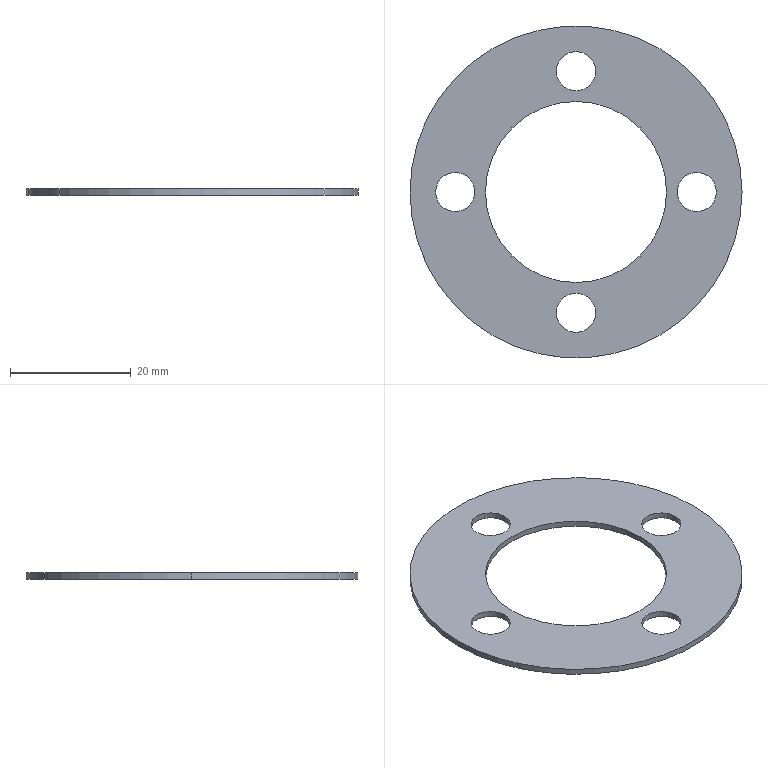Part | SolidWorks | features Extrusion 1 | 1 solid | 14 faces | box 55 x 55 x 1 mm | volume 1536 mm3 | cylinder 12 | plane 2 | commonest cylinder face diameters 6.5 x8 30 x2 55 x2
STEP:
#1=CARTESIAN_POINT('',(-23.25,0.,1.));
#2=VERTEX_POINT('',#1);
#3=CARTESIAN_POINT('',(-16.75,0.,1.));
#4=VERTEX_POINT('',#3);
#5=CARTESIAN_POINT('',(-20.,0.,1.));
#6=DIRECTION('',(0.,0.,1.));
#7=DIRECTION('',(1.,0.,0.));
#8=AXIS2_PLACEMENT_3D('',#5,#6,#7);
#9=CIRCLE('',#8,3.25);
#10=EDGE_CURVE('',#2,#4,#9,.T.);
#11=ORIENTED_EDGE('',*,*,#10,.T.);
#12=CARTESIAN_POINT('',(-16.75,0.,0.));
#13=VERTEX_POINT('',#12);
#14=CARTESIAN_POINT('',(-16.75,0.,1.));
#15=DIRECTION('',(0.,0.,-1.));
#16=VECTOR('',#15,1000.);
#17=LINE('',#14,#16);
#18=EDGE_CURVE('',#4,#13,#17,.T.);
#19=ORIENTED_EDGE('',*,*,#18,.T.);
#20=CARTESIAN_POINT('',(-23.25,0.,0.));
#21=VERTEX_POINT('',#20);
#22=CARTESIAN_POINT('',(-20.,0.,0.));
#23=DIRECTION('',(0.,0.,1.));
#24=DIRECTION('',(1.,0.,0.));
#25=AXIS2_PLACEMENT_3D('',#22,#23,#24);
#26=CIRCLE('',#25,3.25);
#27=EDGE_CURVE('',#21,#13,#26,.T.);
#28=ORIENTED_EDGE('',*,*,#27,.F.);
#29=CARTESIAN_POINT('',(-23.25,0.,1.));
#30=DIRECTION('',(0.,0.,-1.));
#31=VECTOR('',#30,1000.);
#32=LINE('',#29,#31);
#33=EDGE_CURVE('',#2,#21,#32,.T.);
#34=ORIENTED_EDGE('',*,*,#33,.F.);
#35=EDGE_LOOP('',(#11,#19,#28,#34));
#36=FACE_OUTER_BOUND('',#35,.T.);
#37=CARTESIAN_POINT('',(-20.,0.,1.));
#38=DIRECTION('',(0.,0.,-1.));
#39=DIRECTION('',(-1.,0.,0.));
#40=AXIS2_PLACEMENT_3D('',#37,#38,#39);
#41=CYLINDRICAL_SURFACE('',#40,3.25);
#42=ADVANCED_FACE('',(#36),#41,.F.);
#43=CARTESIAN_POINT('',(-3.25,-20.,1.));
#44=VERTEX_POINT('',#43);
#45=CARTESIAN_POINT('',(3.25,-20.,1.));
#46=VERTEX_POINT('',#45);
#47=CARTESIAN_POINT('',(0.,-20.,1.));
#48=DIRECTION('',(0.,0.,1.));
#49=DIRECTION('',(1.,0.,0.));
#50=AXIS2_PLACEMENT_3D('',#47,#48,#49);
#51=CIRCLE('',#50,3.25);
#52=EDGE_CURVE('',#44,#46,#51,.T.);
#53=ORIENTED_EDGE('',*,*,#52,.T.);
#54=CARTESIAN_POINT('',(3.25,-20.,0.));
#55=VERTEX_POINT('',#54);
#56=CARTESIAN_POINT('',(3.25,-20.,1.));
#57=DIRECTION('',(0.,0.,-1.));
#58=VECTOR('',#57,1000.);
#59=LINE('',#56,#58);
#60=EDGE_CURVE('',#46,#55,#59,.T.);
#61=ORIENTED_EDGE('',*,*,#60,.T.);
#62=CARTESIAN_POINT('',(-3.25,-20.,0.));
#63=VERTEX_POINT('',#62);
#64=CARTESIAN_POINT('',(0.,-20.,0.));
#65=DIRECTION('',(0.,0.,1.));
#66=DIRECTION('',(1.,0.,0.));
#67=AXIS2_PLACEMENT_3D('',#64,#65,#66);
#68=CIRCLE('',#67,3.25);
#69=EDGE_CURVE('',#63,#55,#68,.T.);
#70=ORIENTED_EDGE('',*,*,#69,.F.);
#71=CARTESIAN_POINT('',(-3.25,-20.,1.));
#72=DIRECTION('',(0.,0.,-1.));
#73=VECTOR('',#72,1000.);
#74=LINE('',#71,#73);
#75=EDGE_CURVE('',#44,#63,#74,.T.);
#76=ORIENTED_EDGE('',*,*,#75,.F.);
#77=EDGE_LOOP('',(#53,#61,#70,#76));
#78=FACE_OUTER_BOUND('',#77,.T.);
#79=CARTESIAN_POINT('',(0.,-20.,1.));
#80=DIRECTION('',(0.,0.,-1.));
#81=DIRECTION('',(-1.,0.,0.));
#82=AXIS2_PLACEMENT_3D('',#79,#80,#81);
#83=CYLINDRICAL_SURFACE('',#82,3.25);
#84=ADVANCED_FACE('',(#78),#83,.F.);
#85=CARTESIAN_POINT('',(16.75,0.,1.));
#86=VERTEX_POINT('',#85);
#87=CARTESIAN_POINT('',(23.25,0.,1.));
#88=VERTEX_POINT('',#87);
#89=CARTESIAN_POINT('',(20.,0.,1.));
#90=DIRECTION('',(0.,0.,1.));
#91=DIRECTION('',(1.,0.,0.));
#92=AXIS2_PLACEMENT_3D('',#89,#90,#91);
#93=CIRCLE('',#92,3.25);
#94=EDGE_CURVE('',#86,#88,#93,.T.);
#95=ORIENTED_EDGE('',*,*,#94,.T.);
#96=CARTESIAN_POINT('',(23.25,0.,0.));
#97=VERTEX_POINT('',#96);
#98=CARTESIAN_POINT('',(23.25,0.,1.));
#99=DIRECTION('',(0.,0.,-1.));
#100=VECTOR('',#99,1000.);
#101=LINE('',#98,#100);
#102=EDGE_CURVE('',#88,#97,#101,.T.);
#103=ORIENTED_EDGE('',*,*,#102,.T.);
#104=CARTESIAN_POINT('',(16.75,0.,0.));
#105=VERTEX_POINT('',#104);
#106=CARTESIAN_POINT('',(20.,0.,0.));
#107=DIRECTION('',(0.,0.,1.));
#108=DIRECTION('',(1.,0.,0.));
#109=AXIS2_PLACEMENT_3D('',#106,#107,#108);
#110=CIRCLE('',#109,3.25);
#111=EDGE_CURVE('',#105,#97,#110,.T.);
#112=ORIENTED_EDGE('',*,*,#111,.F.);
#113=CARTESIAN_POINT('',(16.75,0.,1.));
#114=DIRECTION('',(0.,0.,-1.));
#115=VECTOR('',#114,1000.);
#116=LINE('',#113,#115);
#117=EDGE_CURVE('',#86,#105,#116,.T.);
#118=ORIENTED_EDGE('',*,*,#117,.F.);
#119=EDGE_LOOP('',(#95,#103,#112,#118));
#120=FACE_OUTER_BOUND('',#119,.T.);
#121=CARTESIAN_POINT('',(20.,0.,1.));
#122=DIRECTION('',(0.,0.,-1.));
#123=DIRECTION('',(-1.,0.,0.));
#124=AXIS2_PLACEMENT_3D('',#121,#122,#123);
#125=CYLINDRICAL_SURFACE('',#124,3.25);
#126=ADVANCED_FACE('',(#120),#125,.F.);
#127=CARTESIAN_POINT('',(-3.25,20.,1.));
#128=VERTEX_POINT('',#127);
#129=CARTESIAN_POINT('',(3.25,20.,1.));
#130=VERTEX_POINT('',#129);
#131=CARTESIAN_POINT('',(0.,20.,1.));
#132=DIRECTION('',(0.,0.,1.));
#133=DIRECTION('',(1.,0.,0.));
#134=AXIS2_PLACEMENT_3D('',#131,#132,#133);
#135=CIRCLE('',#134,3.25);
#136=EDGE_CURVE('',#128,#130,#135,.T.);
#137=ORIENTED_EDGE('',*,*,#136,.T.);
#138=CARTESIAN_POINT('',(3.25,20.,0.));
#139=VERTEX_POINT('',#138);
#140=CARTESIAN_POINT('',(3.25,20.,1.));
#141=DIRECTION('',(0.,0.,-1.));
#142=VECTOR('',#141,1000.);
#143=LINE('',#140,#142);
#144=EDGE_CURVE('',#130,#139,#143,.T.);
#145=ORIENTED_EDGE('',*,*,#144,.T.);
#146=CARTESIAN_POINT('',(-3.25,20.,0.));
#147=VERTEX_POINT('',#146);
#148=CARTESIAN_POINT('',(0.,20.,0.));
#149=DIRECTION('',(0.,0.,1.));
#150=DIRECTION('',(1.,0.,0.));
#151=AXIS2_PLACEMENT_3D('',#148,#149,#150);
#152=CIRCLE('',#151,3.25);
#153=EDGE_CURVE('',#147,#139,#152,.T.);
#154=ORIENTED_EDGE('',*,*,#153,.F.);
#155=CARTESIAN_POINT('',(-3.25,20.,1.));
#156=DIRECTION('',(0.,0.,-1.));
#157=VECTOR('',#156,1000.);
#158=LINE('',#155,#157);
#159=EDGE_CURVE('',#128,#147,#158,.T.);
#160=ORIENTED_EDGE('',*,*,#159,.F.);
#161=EDGE_LOOP('',(#137,#145,#154,#160));
#162=FACE_OUTER_BOUND('',#161,.T.);
#163=CARTESIAN_POINT('',(0.,20.,1.));
#164=DIRECTION('',(0.,0.,-1.));
#165=DIRECTION('',(-1.,0.,0.));
#166=AXIS2_PLACEMENT_3D('',#163,#164,#165);
#167=CYLINDRICAL_SURFACE('',#166,3.25);
#168=ADVANCED_FACE('',(#162),#167,.F.);
#169=CARTESIAN_POINT('',(-15.,0.,1.));
#170=VERTEX_POINT('',#169);
#171=CARTESIAN_POINT('',(15.,0.,1.));
#172=VERTEX_POINT('',#171);
#173=CARTESIAN_POINT('',(0.,0.,1.));
#174=DIRECTION('',(0.,0.,1.));
#175=DIRECTION('',(1.,0.,0.));
#176=AXIS2_PLACEMENT_3D('',#173,#174,#175);
#177=CIRCLE('',#176,15.);
#178=EDGE_CURVE('',#170,#172,#177,.T.);
#179=ORIENTED_EDGE('',*,*,#178,.T.);
#180=CARTESIAN_POINT('',(15.,0.,0.));
#181=VERTEX_POINT('',#180);
#182=CARTESIAN_POINT('',(15.,0.,1.));
#183=DIRECTION('',(0.,0.,-1.));
#184=VECTOR('',#183,1000.);
#185=LINE('',#182,#184);
#186=EDGE_CURVE('',#172,#181,#185,.T.);
#187=ORIENTED_EDGE('',*,*,#186,.T.);
#188=CARTESIAN_POINT('',(-15.,0.,0.));
#189=VERTEX_POINT('',#188);
#190=CARTESIAN_POINT('',(0.,0.,0.));
#191=DIRECTION('',(0.,0.,1.));
#192=DIRECTION('',(1.,0.,0.));
#193=AXIS2_PLACEMENT_3D('',#190,#191,#192);
#194=CIRCLE('',#193,15.);
#195=EDGE_CURVE('',#189,#181,#194,.T.);
#196=ORIENTED_EDGE('',*,*,#195,.F.);
#197=CARTESIAN_POINT('',(-15.,0.,1.));
#198=DIRECTION('',(0.,0.,-1.));
#199=VECTOR('',#198,1000.);
#200=LINE('',#197,#199);
#201=EDGE_CURVE('',#170,#189,#200,.T.);
#202=ORIENTED_EDGE('',*,*,#201,.F.);
#203=EDGE_LOOP('',(#179,#187,#196,#202));
#204=FACE_OUTER_BOUND('',#203,.T.);
#205=CARTESIAN_POINT('',(0.,0.,1.));
#206=DIRECTION('',(0.,0.,-1.));
#207=DIRECTION('',(-1.,0.,0.));
#208=AXIS2_PLACEMENT_3D('',#205,#206,#207);
#209=CYLINDRICAL_SURFACE('',#208,15.);
#210=ADVANCED_FACE('',(#204),#209,.F.);
#211=CARTESIAN_POINT('',(27.5,0.,1.));
#212=VERTEX_POINT('',#211);
#213=CARTESIAN_POINT('',(-27.5,0.,1.));
#214=VERTEX_POINT('',#213);
#215=CARTESIAN_POINT('',(0.,0.,1.));
#216=DIRECTION('',(0.,0.,1.));
#217=DIRECTION('',(1.,0.,0.));
#218=AXIS2_PLACEMENT_3D('',#215,#216,#217);
#219=CIRCLE('',#218,27.5);
#220=EDGE_CURVE('',#212,#214,#219,.T.);
#221=ORIENTED_EDGE('',*,*,#220,.F.);
#222=CARTESIAN_POINT('',(27.5,0.,0.));
#223=VERTEX_POINT('',#222);
#224=CARTESIAN_POINT('',(27.5,0.,1.));
#225=DIRECTION('',(0.,0.,-1.));
#226=VECTOR('',#225,1000.);
#227=LINE('',#224,#226);
#228=EDGE_CURVE('',#212,#223,#227,.T.);
#229=ORIENTED_EDGE('',*,*,#228,.T.);
#230=CARTESIAN_POINT('',(-27.5,0.,0.));
#231=VERTEX_POINT('',#230);
#232=CARTESIAN_POINT('',(0.,0.,0.));
#233=DIRECTION('',(0.,0.,1.));
#234=DIRECTION('',(1.,0.,0.));
#235=AXIS2_PLACEMENT_3D('',#232,#233,#234);
#236=CIRCLE('',#235,27.5);
#237=EDGE_CURVE('',#223,#231,#236,.T.);
#238=ORIENTED_EDGE('',*,*,#237,.T.);
#239=CARTESIAN_POINT('',(-27.5,0.,1.));
#240=DIRECTION('',(0.,0.,-1.));
#241=VECTOR('',#240,1000.);
#242=LINE('',#239,#241);
#243=EDGE_CURVE('',#214,#231,#242,.T.);
#244=ORIENTED_EDGE('',*,*,#243,.F.);
#245=EDGE_LOOP('',(#221,#229,#238,#244));
#246=FACE_OUTER_BOUND('',#245,.T.);
#247=CARTESIAN_POINT('',(0.,0.,1.));
#248=DIRECTION('',(0.,0.,-1.));
#249=DIRECTION('',(-1.,0.,0.));
#250=AXIS2_PLACEMENT_3D('',#247,#248,#249);
#251=CYLINDRICAL_SURFACE('',#250,27.5);
#252=ADVANCED_FACE('',(#246),#251,.T.);
#253=ORIENTED_EDGE('',*,*,#52,.F.);
#254=CARTESIAN_POINT('',(0.,-20.,1.));
#255=DIRECTION('',(0.,0.,1.));
#256=DIRECTION('',(1.,0.,0.));
#257=AXIS2_PLACEMENT_3D('',#254,#255,#256);
#258=CIRCLE('',#257,3.25);
#259=EDGE_CURVE('',#46,#44,#258,.T.);
#260=ORIENTED_EDGE('',*,*,#259,.F.);
#261=EDGE_LOOP('',(#253,#260));
#262=FACE_BOUND('',#261,.T.);
#263=ORIENTED_EDGE('',*,*,#136,.F.);
#264=CARTESIAN_POINT('',(0.,20.,1.));
#265=DIRECTION('',(0.,0.,1.));
#266=DIRECTION('',(1.,0.,0.));
#267=AXIS2_PLACEMENT_3D('',#264,#265,#266);
#268=CIRCLE('',#267,3.25);
#269=EDGE_CURVE('',#130,#128,#268,.T.);
#270=ORIENTED_EDGE('',*,*,#269,.F.);
#271=EDGE_LOOP('',(#263,#270));
#272=FACE_BOUND('',#271,.T.);
#273=CARTESIAN_POINT('',(0.,0.,1.));
#274=DIRECTION('',(0.,0.,1.));
#275=DIRECTION('',(1.,0.,0.));
#276=AXIS2_PLACEMENT_3D('',#273,#274,#275);
#277=CIRCLE('',#276,27.5);
#278=EDGE_CURVE('',#214,#212,#277,.T.);
#279=ORIENTED_EDGE('',*,*,#278,.T.);
#280=ORIENTED_EDGE('',*,*,#220,.T.);
#281=EDGE_LOOP('',(#279,#280));
#282=FACE_OUTER_BOUND('',#281,.T.);
#283=ORIENTED_EDGE('',*,*,#178,.F.);
#284=CARTESIAN_POINT('',(0.,0.,1.));
#285=DIRECTION('',(0.,0.,1.));
#286=DIRECTION('',(1.,0.,0.));
#287=AXIS2_PLACEMENT_3D('',#284,#285,#286);
#288=CIRCLE('',#287,15.);
#289=EDGE_CURVE('',#172,#170,#288,.T.);
#290=ORIENTED_EDGE('',*,*,#289,.F.);
#291=EDGE_LOOP('',(#283,#290));
#292=FACE_BOUND('',#291,.T.);
#293=ORIENTED_EDGE('',*,*,#94,.F.);
#294=CARTESIAN_POINT('',(20.,0.,1.));
#295=DIRECTION('',(0.,0.,1.));
#296=DIRECTION('',(1.,0.,0.));
#297=AXIS2_PLACEMENT_3D('',#294,#295,#296);
#298=CIRCLE('',#297,3.25);
#299=EDGE_CURVE('',#88,#86,#298,.T.);
#300=ORIENTED_EDGE('',*,*,#299,.F.);
#301=EDGE_LOOP('',(#293,#300));
#302=FACE_BOUND('',#301,.T.);
#303=ORIENTED_EDGE('',*,*,#10,.F.);
#304=CARTESIAN_POINT('',(-20.,0.,1.));
#305=DIRECTION('',(0.,0.,1.));
#306=DIRECTION('',(1.,0.,0.));
#307=AXIS2_PLACEMENT_3D('',#304,#305,#306);
#308=CIRCLE('',#307,3.25);
#309=EDGE_CURVE('',#4,#2,#308,.T.);
#310=ORIENTED_EDGE('',*,*,#309,.F.);
#311=EDGE_LOOP('',(#303,#310));
#312=FACE_BOUND('',#311,.T.);
#313=CARTESIAN_POINT('',(0.,0.,1.));
#314=DIRECTION('',(0.,0.,1.));
#315=DIRECTION('',(1.,0.,0.));
#316=AXIS2_PLACEMENT_3D('',#313,#314,#315);
#317=PLANE('',#316);
#318=ADVANCED_FACE('',(#262,#272,#282,#292,#302,#312),#317,.T.);
#319=CARTESIAN_POINT('',(0.,0.,0.));
#320=DIRECTION('',(0.,0.,1.));
#321=DIRECTION('',(1.,0.,0.));
#322=AXIS2_PLACEMENT_3D('',#319,#320,#321);
#323=CIRCLE('',#322,27.5);
#324=EDGE_CURVE('',#231,#223,#323,.T.);
#325=ORIENTED_EDGE('',*,*,#324,.F.);
#326=ORIENTED_EDGE('',*,*,#237,.F.);
#327=EDGE_LOOP('',(#325,#326));
#328=FACE_OUTER_BOUND('',#327,.T.);
#329=ORIENTED_EDGE('',*,*,#195,.T.);
#330=CARTESIAN_POINT('',(0.,0.,0.));
#331=DIRECTION('',(0.,0.,1.));
#332=DIRECTION('',(1.,0.,0.));
#333=AXIS2_PLACEMENT_3D('',#330,#331,#332);
#334=CIRCLE('',#333,15.);
#335=EDGE_CURVE('',#181,#189,#334,.T.);
#336=ORIENTED_EDGE('',*,*,#335,.T.);
#337=EDGE_LOOP('',(#329,#336));
#338=FACE_BOUND('',#337,.T.);
#339=ORIENTED_EDGE('',*,*,#153,.T.);
#340=CARTESIAN_POINT('',(0.,20.,0.));
#341=DIRECTION('',(0.,0.,1.));
#342=DIRECTION('',(1.,0.,0.));
#343=AXIS2_PLACEMENT_3D('',#340,#341,#342);
#344=CIRCLE('',#343,3.25);
#345=EDGE_CURVE('',#139,#147,#344,.T.);
#346=ORIENTED_EDGE('',*,*,#345,.T.);
#347=EDGE_LOOP('',(#339,#346));
#348=FACE_BOUND('',#347,.T.);
#349=ORIENTED_EDGE('',*,*,#111,.T.);
#350=CARTESIAN_POINT('',(20.,0.,0.));
#351=DIRECTION('',(0.,0.,1.));
#352=DIRECTION('',(1.,0.,0.));
#353=AXIS2_PLACEMENT_3D('',#350,#351,#352);
#354=CIRCLE('',#353,3.25);
#355=EDGE_CURVE('',#97,#105,#354,.T.);
#356=ORIENTED_EDGE('',*,*,#355,.T.);
#357=EDGE_LOOP('',(#349,#356));
#358=FACE_BOUND('',#357,.T.);
#359=ORIENTED_EDGE('',*,*,#69,.T.);
#360=CARTESIAN_POINT('',(0.,-20.,0.));
#361=DIRECTION('',(0.,0.,1.));
#362=DIRECTION('',(1.,0.,0.));
#363=AXIS2_PLACEMENT_3D('',#360,#361,#362);
#364=CIRCLE('',#363,3.25);
#365=EDGE_CURVE('',#55,#63,#364,.T.);
#366=ORIENTED_EDGE('',*,*,#365,.T.);
#367=EDGE_LOOP('',(#359,#366));
#368=FACE_BOUND('',#367,.T.);
#369=ORIENTED_EDGE('',*,*,#27,.T.);
#370=CARTESIAN_POINT('',(-20.,0.,0.));
#371=DIRECTION('',(0.,0.,1.));
#372=DIRECTION('',(1.,0.,0.));
#373=AXIS2_PLACEMENT_3D('',#370,#371,#372);
#374=CIRCLE('',#373,3.25);
#375=EDGE_CURVE('',#13,#21,#374,.T.);
#376=ORIENTED_EDGE('',*,*,#375,.T.);
#377=EDGE_LOOP('',(#369,#376));
#378=FACE_BOUND('',#377,.T.);
#379=CARTESIAN_POINT('',(0.,0.,0.));
#380=DIRECTION('',(0.,0.,1.));
#381=DIRECTION('',(1.,0.,0.));
#382=AXIS2_PLACEMENT_3D('',#379,#380,#381);
#383=PLANE('',#382);
#384=ADVANCED_FACE('',(#328,#338,#348,#358,#368,#378),#383,.F.);
#385=ORIENTED_EDGE('',*,*,#228,.F.);
#386=ORIENTED_EDGE('',*,*,#278,.F.);
#387=ORIENTED_EDGE('',*,*,#243,.T.);
#388=ORIENTED_EDGE('',*,*,#324,.T.);
#389=EDGE_LOOP('',(#385,#386,#387,#388));
#390=FACE_OUTER_BOUND('',#389,.T.);
#391=CARTESIAN_POINT('',(0.,0.,1.));
#392=DIRECTION('',(0.,0.,-1.));
#393=DIRECTION('',(-1.,0.,0.));
#394=AXIS2_PLACEMENT_3D('',#391,#392,#393);
#395=CYLINDRICAL_SURFACE('',#394,27.5);
#396=ADVANCED_FACE('',(#390),#395,.T.);
#397=ORIENTED_EDGE('',*,*,#186,.F.);
#398=ORIENTED_EDGE('',*,*,#289,.T.);
#399=ORIENTED_EDGE('',*,*,#201,.T.);
#400=ORIENTED_EDGE('',*,*,#335,.F.);
#401=EDGE_LOOP('',(#397,#398,#399,#400));
#402=FACE_OUTER_BOUND('',#401,.T.);
#403=CARTESIAN_POINT('',(0.,0.,1.));
#404=DIRECTION('',(0.,0.,-1.));
#405=DIRECTION('',(-1.,0.,0.));
#406=AXIS2_PLACEMENT_3D('',#403,#404,#405);
#407=CYLINDRICAL_SURFACE('',#406,15.);
#408=ADVANCED_FACE('',(#402),#407,.F.);
#409=ORIENTED_EDGE('',*,*,#144,.F.);
#410=ORIENTED_EDGE('',*,*,#269,.T.);
#411=ORIENTED_EDGE('',*,*,#159,.T.);
#412=ORIENTED_EDGE('',*,*,#345,.F.);
#413=EDGE_LOOP('',(#409,#410,#411,#412));
#414=FACE_OUTER_BOUND('',#413,.T.);
#415=CARTESIAN_POINT('',(0.,20.,1.));
#416=DIRECTION('',(0.,0.,-1.));
#417=DIRECTION('',(-1.,0.,0.));
#418=AXIS2_PLACEMENT_3D('',#415,#416,#417);
#419=CYLINDRICAL_SURFACE('',#418,3.25);
#420=ADVANCED_FACE('',(#414),#419,.F.);
#421=ORIENTED_EDGE('',*,*,#102,.F.);
#422=ORIENTED_EDGE('',*,*,#299,.T.);
#423=ORIENTED_EDGE('',*,*,#117,.T.);
#424=ORIENTED_EDGE('',*,*,#355,.F.);
#425=EDGE_LOOP('',(#421,#422,#423,#424));
#426=FACE_OUTER_BOUND('',#425,.T.);
#427=CARTESIAN_POINT('',(20.,0.,1.));
#428=DIRECTION('',(0.,0.,-1.));
#429=DIRECTION('',(-1.,0.,0.));
#430=AXIS2_PLACEMENT_3D('',#427,#428,#429);
#431=CYLINDRICAL_SURFACE('',#430,3.25);
#432=ADVANCED_FACE('',(#426),#431,.F.);
#433=ORIENTED_EDGE('',*,*,#60,.F.);
#434=ORIENTED_EDGE('',*,*,#259,.T.);
#435=ORIENTED_EDGE('',*,*,#75,.T.);
#436=ORIENTED_EDGE('',*,*,#365,.F.);
#437=EDGE_LOOP('',(#433,#434,#435,#436));
#438=FACE_OUTER_BOUND('',#437,.T.);
#439=CARTESIAN_POINT('',(0.,-20.,1.));
#440=DIRECTION('',(0.,0.,-1.));
#441=DIRECTION('',(-1.,0.,0.));
#442=AXIS2_PLACEMENT_3D('',#439,#440,#441);
#443=CYLINDRICAL_SURFACE('',#442,3.25);
#444=ADVANCED_FACE('',(#438),#443,.F.);
#445=ORIENTED_EDGE('',*,*,#18,.F.);
#446=ORIENTED_EDGE('',*,*,#309,.T.);
#447=ORIENTED_EDGE('',*,*,#33,.T.);
#448=ORIENTED_EDGE('',*,*,#375,.F.);
#449=EDGE_LOOP('',(#445,#446,#447,#448));
#450=FACE_OUTER_BOUND('',#449,.T.);
#451=CARTESIAN_POINT('',(-20.,0.,1.));
#452=DIRECTION('',(0.,0.,-1.));
#453=DIRECTION('',(-1.,0.,0.));
#454=AXIS2_PLACEMENT_3D('',#451,#452,#453);
#455=CYLINDRICAL_SURFACE('',#454,3.25);
#456=ADVANCED_FACE('',(#450),#455,.F.);
#457=CLOSED_SHELL('',(#42,#84,#126,#168,#210,#252,#318,#384,#396,#408,#420,#432,#444,#456));
#458=MANIFOLD_SOLID_BREP('',#457);
#459=CARTESIAN_POINT('',(0.,0.,0.));
#460=DIRECTION('',(0.,0.,1.));
#461=DIRECTION('',(1.,0.,0.));
#462=AXIS2_PLACEMENT_3D('',#459,#460,#461);
#463=(LENGTH_UNIT()NAMED_UNIT(*)SI_UNIT(.MILLI.,.METRE.));
#464=UNCERTAINTY_MEASURE_WITH_UNIT(LENGTH_MEASURE(0.00001),#463,'','');
#465=(NAMED_UNIT(*)PLANE_ANGLE_UNIT()SI_UNIT($,.RADIAN.));
#466=(NAMED_UNIT(*)SI_UNIT($,.STERADIAN.)SOLID_ANGLE_UNIT());
#467=(GEOMETRIC_REPRESENTATION_CONTEXT(3)GLOBAL_UNCERTAINTY_ASSIGNED_CONTEXT((#464))GLOBAL_UNIT_ASSIGNED_CONTEXT((#463,#465,#466))REPRESENTATION_CONTEXT('',''));
#468=ADVANCED_BREP_SHAPE_REPRESENTATION('',(#458,#462),#467);